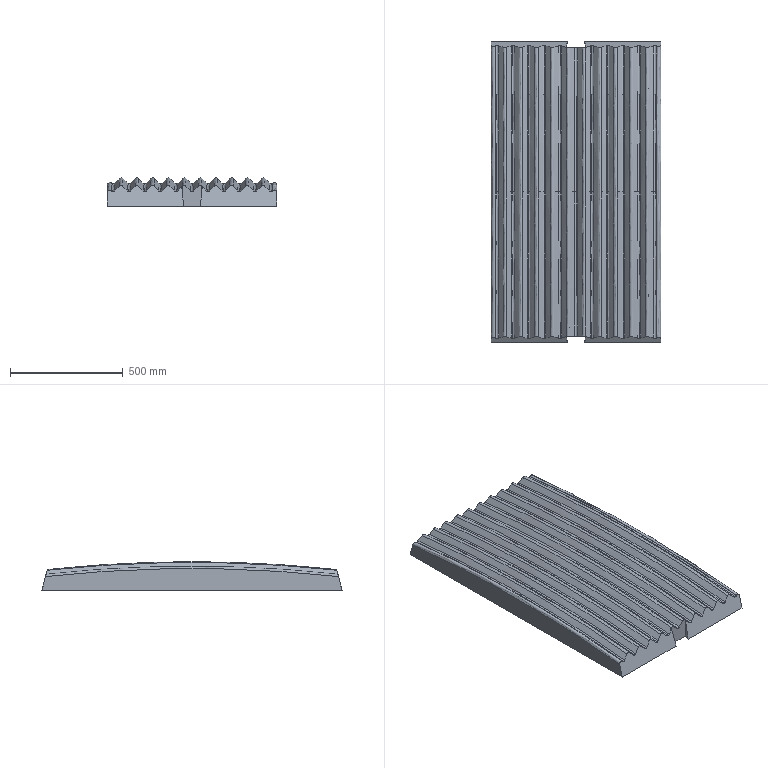Part | SolidWorks | features ICE 4, LPattern 2, MirrorPattern 2, Extrusion 1, Fillet 1, SweepCut 1 | 1 solid | 162 faces | box 750 x 1330 x 125.858 mm | volume 65171136 mm3 | plane 63 | torus 56 | cone 33 | cylinder 10 | commonest cylinder face diameters 11860 x10